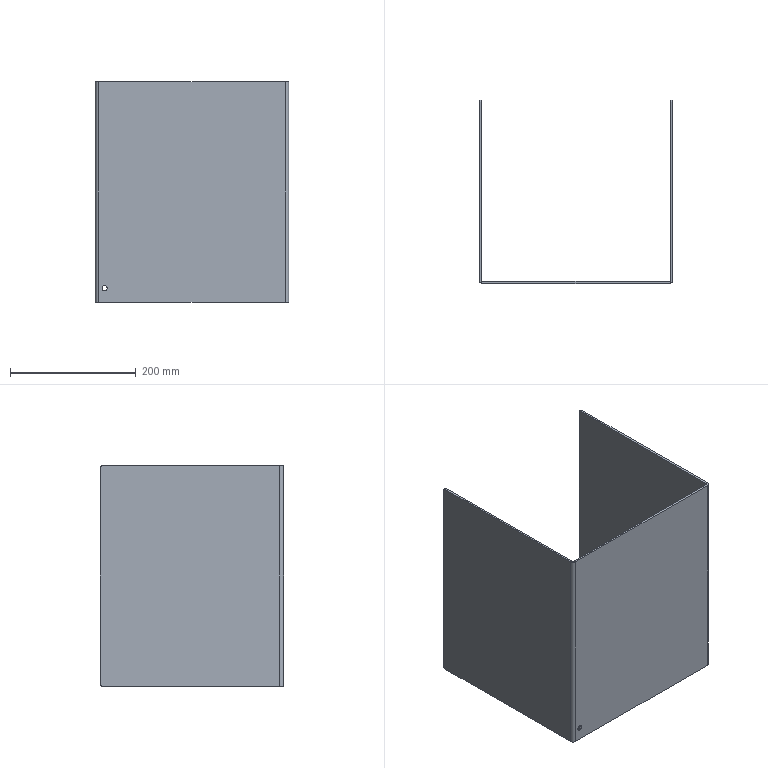Part | SolidWorks | features ICE 2, FlatPattern 1, SMBaseFlange 1, SheetMetal 1 | 1 solid | 28 faces | box 308 x 291 x 350 mm | volume 923970 mm3 | plane 18 | cylinder 10 | commonest cylinder face diameters 6 x6 8 x2 12 x2
STEP:
#1=CARTESIAN_POINT('',(15.,3.,-324.));
#2=VERTEX_POINT('',#1);
#3=CARTESIAN_POINT('',(15.,3.,-332.));
#4=VERTEX_POINT('',#3);
#5=CARTESIAN_POINT('',(15.,3.,-328.));
#6=DIRECTION('',(0.,-1.,0.));
#7=DIRECTION('',(0.,0.,-1.));
#8=AXIS2_PLACEMENT_3D('',#5,#6,#7);
#9=CIRCLE('',#8,4.);
#10=EDGE_CURVE('',#2,#4,#9,.T.);
#11=ORIENTED_EDGE('',*,*,#10,.F.);
#12=CARTESIAN_POINT('',(15.,0.,-324.));
#13=VERTEX_POINT('',#12);
#14=CARTESIAN_POINT('',(15.,10.,-324.));
#15=DIRECTION('',(0.,-1.,0.));
#16=VECTOR('',#15,1000.);
#17=LINE('',#14,#16);
#18=EDGE_CURVE('',#2,#13,#17,.T.);
#19=ORIENTED_EDGE('',*,*,#18,.T.);
#20=CARTESIAN_POINT('',(15.,0.,-332.));
#21=VERTEX_POINT('',#20);
#22=CARTESIAN_POINT('',(15.,0.,-328.));
#23=DIRECTION('',(0.,-1.,0.));
#24=DIRECTION('',(0.,0.,-1.));
#25=AXIS2_PLACEMENT_3D('',#22,#23,#24);
#26=CIRCLE('',#25,4.);
#27=EDGE_CURVE('',#13,#21,#26,.T.);
#28=ORIENTED_EDGE('',*,*,#27,.T.);
#29=CARTESIAN_POINT('',(15.,10.,-332.));
#30=DIRECTION('',(0.,-1.,0.));
#31=VECTOR('',#30,1000.);
#32=LINE('',#29,#31);
#33=EDGE_CURVE('',#4,#21,#32,.T.);
#34=ORIENTED_EDGE('',*,*,#33,.F.);
#35=EDGE_LOOP('',(#11,#19,#28,#34));
#36=FACE_OUTER_BOUND('',#35,.T.);
#37=CARTESIAN_POINT('',(15.,10.,-328.));
#38=DIRECTION('',(0.,-1.,0.));
#39=DIRECTION('',(0.,0.,-1.));
#40=AXIS2_PLACEMENT_3D('',#37,#38,#39);
#41=CYLINDRICAL_SURFACE('',#40,4.);
#42=ADVANCED_FACE('',(#36),#41,.F.);
#43=CARTESIAN_POINT('',(0.,288.,0.));
#44=VERTEX_POINT('',#43);
#45=CARTESIAN_POINT('',(0.,6.,0.));
#46=VERTEX_POINT('',#45);
#47=CARTESIAN_POINT('',(0.,0.,0.));
#48=DIRECTION('',(0.,-1.,0.));
#49=VECTOR('',#48,1000.);
#50=LINE('',#47,#49);
#51=EDGE_CURVE('',#44,#46,#50,.T.);
#52=ORIENTED_EDGE('',*,*,#51,.F.);
#53=CARTESIAN_POINT('',(0.,291.,-3.));
#54=VERTEX_POINT('',#53);
#55=CARTESIAN_POINT('',(0.,288.,-3.));
#56=DIRECTION('',(1.,0.,0.));
#57=DIRECTION('',(0.,0.,1.));
#58=AXIS2_PLACEMENT_3D('',#55,#56,#57);
#59=CIRCLE('',#58,3.);
#60=EDGE_CURVE('',#54,#44,#59,.T.);
#61=ORIENTED_EDGE('',*,*,#60,.F.);
#62=CARTESIAN_POINT('',(0.,291.,-347.));
#63=VERTEX_POINT('',#62);
#64=CARTESIAN_POINT('',(0.,291.,-350.));
#65=DIRECTION('',(0.,0.,1.));
#66=VECTOR('',#65,1000.);
#67=LINE('',#64,#66);
#68=EDGE_CURVE('',#63,#54,#67,.T.);
#69=ORIENTED_EDGE('',*,*,#68,.F.);
#70=CARTESIAN_POINT('',(0.,288.,-350.));
#71=VERTEX_POINT('',#70);
#72=CARTESIAN_POINT('',(0.,288.,-347.));
#73=DIRECTION('',(1.,0.,0.));
#74=DIRECTION('',(0.,0.,1.));
#75=AXIS2_PLACEMENT_3D('',#72,#73,#74);
#76=CIRCLE('',#75,3.);
#77=EDGE_CURVE('',#71,#63,#76,.T.);
#78=ORIENTED_EDGE('',*,*,#77,.F.);
#79=CARTESIAN_POINT('',(0.,6.,-350.));
#80=VERTEX_POINT('',#79);
#81=CARTESIAN_POINT('',(0.,0.,-350.));
#82=DIRECTION('',(0.,-1.,0.));
#83=VECTOR('',#82,1000.);
#84=LINE('',#81,#83);
#85=EDGE_CURVE('',#71,#80,#84,.T.);
#86=ORIENTED_EDGE('',*,*,#85,.T.);
#87=CARTESIAN_POINT('',(0.,6.,-350.));
#88=DIRECTION('',(0.,0.,1.));
#89=VECTOR('',#88,1000.);
#90=LINE('',#87,#89);
#91=EDGE_CURVE('',#80,#46,#90,.T.);
#92=ORIENTED_EDGE('',*,*,#91,.T.);
#93=EDGE_LOOP('',(#52,#61,#69,#78,#86,#92));
#94=FACE_OUTER_BOUND('',#93,.T.);
#95=CARTESIAN_POINT('',(0.,0.,-350.));
#96=DIRECTION('',(-1.,0.,0.));
#97=DIRECTION('',(0.,0.,1.));
#98=AXIS2_PLACEMENT_3D('',#95,#96,#97);
#99=PLANE('',#98);
#100=ADVANCED_FACE('',(#94),#99,.T.);
#101=CARTESIAN_POINT('',(3.,291.,-3.));
#102=VERTEX_POINT('',#101);
#103=CARTESIAN_POINT('',(3.,288.,0.));
#104=VERTEX_POINT('',#103);
#105=CARTESIAN_POINT('',(3.,288.,-3.));
#106=DIRECTION('',(1.,0.,0.));
#107=DIRECTION('',(0.,0.,1.));
#108=AXIS2_PLACEMENT_3D('',#105,#106,#107);
#109=CIRCLE('',#108,3.);
#110=EDGE_CURVE('',#102,#104,#109,.T.);
#111=ORIENTED_EDGE('',*,*,#110,.T.);
#112=CARTESIAN_POINT('',(3.,6.,0.));
#113=VERTEX_POINT('',#112);
#114=CARTESIAN_POINT('',(3.,0.,0.));
#115=DIRECTION('',(0.,-1.,0.));
#116=VECTOR('',#115,1000.);
#117=LINE('',#114,#116);
#118=EDGE_CURVE('',#104,#113,#117,.T.);
#119=ORIENTED_EDGE('',*,*,#118,.T.);
#120=CARTESIAN_POINT('',(3.,6.,-350.));
#121=VERTEX_POINT('',#120);
#122=CARTESIAN_POINT('',(3.,6.,-350.));
#123=DIRECTION('',(0.,0.,1.));
#124=VECTOR('',#123,1000.);
#125=LINE('',#122,#124);
#126=EDGE_CURVE('',#121,#113,#125,.T.);
#127=ORIENTED_EDGE('',*,*,#126,.F.);
#128=CARTESIAN_POINT('',(3.,288.,-350.));
#129=VERTEX_POINT('',#128);
#130=CARTESIAN_POINT('',(3.,0.,-350.));
#131=DIRECTION('',(0.,-1.,0.));
#132=VECTOR('',#131,1000.);
#133=LINE('',#130,#132);
#134=EDGE_CURVE('',#129,#121,#133,.T.);
#135=ORIENTED_EDGE('',*,*,#134,.F.);
#136=CARTESIAN_POINT('',(3.,291.,-347.));
#137=VERTEX_POINT('',#136);
#138=CARTESIAN_POINT('',(3.,288.,-347.));
#139=DIRECTION('',(1.,0.,0.));
#140=DIRECTION('',(0.,0.,1.));
#141=AXIS2_PLACEMENT_3D('',#138,#139,#140);
#142=CIRCLE('',#141,3.);
#143=EDGE_CURVE('',#129,#137,#142,.T.);
#144=ORIENTED_EDGE('',*,*,#143,.T.);
#145=CARTESIAN_POINT('',(3.,291.,-350.));
#146=DIRECTION('',(0.,0.,1.));
#147=VECTOR('',#146,1000.);
#148=LINE('',#145,#147);
#149=EDGE_CURVE('',#137,#102,#148,.T.);
#150=ORIENTED_EDGE('',*,*,#149,.T.);
#151=EDGE_LOOP('',(#111,#119,#127,#135,#144,#150));
#152=FACE_OUTER_BOUND('',#151,.T.);
#153=CARTESIAN_POINT('',(3.,0.,-350.));
#154=DIRECTION('',(-1.,0.,0.));
#155=DIRECTION('',(0.,0.,1.));
#156=AXIS2_PLACEMENT_3D('',#153,#154,#155);
#157=PLANE('',#156);
#158=ADVANCED_FACE('',(#152),#157,.F.);
#159=ORIENTED_EDGE('',*,*,#118,.F.);
#160=CARTESIAN_POINT('',(3.,288.,0.));
#161=DIRECTION('',(-1.,0.,0.));
#162=VECTOR('',#161,1000.);
#163=LINE('',#160,#162);
#164=EDGE_CURVE('',#104,#44,#163,.T.);
#165=ORIENTED_EDGE('',*,*,#164,.T.);
#166=ORIENTED_EDGE('',*,*,#51,.T.);
#167=CARTESIAN_POINT('',(0.,6.,0.));
#168=DIRECTION('',(1.,0.,0.));
#169=VECTOR('',#168,1000.);
#170=LINE('',#167,#169);
#171=EDGE_CURVE('',#46,#113,#170,.T.);
#172=ORIENTED_EDGE('',*,*,#171,.T.);
#173=EDGE_LOOP('',(#159,#165,#166,#172));
#174=FACE_OUTER_BOUND('',#173,.T.);
#175=CARTESIAN_POINT('',(6.,3.,0.));
#176=DIRECTION('',(0.,0.,1.));
#177=DIRECTION('',(1.,0.,0.));
#178=AXIS2_PLACEMENT_3D('',#175,#176,#177);
#179=PLANE('',#178);
#180=ADVANCED_FACE('',(#174),#179,.T.);
#181=CARTESIAN_POINT('',(3.,291.,-3.));
#182=DIRECTION('',(-1.,0.,0.));
#183=VECTOR('',#182,1000.);
#184=LINE('',#181,#183);
#185=EDGE_CURVE('',#102,#54,#184,.T.);
#186=ORIENTED_EDGE('',*,*,#185,.F.);
#187=ORIENTED_EDGE('',*,*,#149,.F.);
#188=CARTESIAN_POINT('',(3.,291.,-347.));
#189=DIRECTION('',(-1.,0.,0.));
#190=VECTOR('',#189,1000.);
#191=LINE('',#188,#190);
#192=EDGE_CURVE('',#137,#63,#191,.T.);
#193=ORIENTED_EDGE('',*,*,#192,.T.);
#194=ORIENTED_EDGE('',*,*,#68,.T.);
#195=EDGE_LOOP('',(#186,#187,#193,#194));
#196=FACE_OUTER_BOUND('',#195,.T.);
#197=CARTESIAN_POINT('',(0.,291.,-350.));
#198=DIRECTION('',(0.,-1.,0.));
#199=DIRECTION('',(0.,0.,-1.));
#200=AXIS2_PLACEMENT_3D('',#197,#198,#199);
#201=PLANE('',#200);
#202=ADVANCED_FACE('',(#196),#201,.F.);
#203=CARTESIAN_POINT('',(308.,291.,-347.));
#204=VERTEX_POINT('',#203);
#205=CARTESIAN_POINT('',(308.,291.,-3.));
#206=VERTEX_POINT('',#205);
#207=CARTESIAN_POINT('',(308.,291.,-350.));
#208=DIRECTION('',(0.,0.,1.));
#209=VECTOR('',#208,1000.);
#210=LINE('',#207,#209);
#211=EDGE_CURVE('',#204,#206,#210,.T.);
#212=ORIENTED_EDGE('',*,*,#211,.T.);
#213=CARTESIAN_POINT('',(308.,288.,0.));
#214=VERTEX_POINT('',#213);
#215=CARTESIAN_POINT('',(308.,288.,-3.));
#216=DIRECTION('',(-1.,0.,0.));
#217=DIRECTION('',(0.,0.,-1.));
#218=AXIS2_PLACEMENT_3D('',#215,#216,#217);
#219=CIRCLE('',#218,3.);
#220=EDGE_CURVE('',#214,#206,#219,.T.);
#221=ORIENTED_EDGE('',*,*,#220,.F.);
#222=CARTESIAN_POINT('',(308.,6.,0.));
#223=VERTEX_POINT('',#222);
#224=CARTESIAN_POINT('',(308.,0.,0.));
#225=DIRECTION('',(0.,1.,0.));
#226=VECTOR('',#225,1000.);
#227=LINE('',#224,#226);
#228=EDGE_CURVE('',#223,#214,#227,.T.);
#229=ORIENTED_EDGE('',*,*,#228,.F.);
#230=CARTESIAN_POINT('',(308.,6.,-350.));
#231=VERTEX_POINT('',#230);
#232=CARTESIAN_POINT('',(308.,6.,-350.));
#233=DIRECTION('',(0.,0.,1.));
#234=VECTOR('',#233,1000.);
#235=LINE('',#232,#234);
#236=EDGE_CURVE('',#231,#223,#235,.T.);
#237=ORIENTED_EDGE('',*,*,#236,.F.);
#238=CARTESIAN_POINT('',(308.,288.,-350.));
#239=VERTEX_POINT('',#238);
#240=CARTESIAN_POINT('',(308.,0.,-350.));
#241=DIRECTION('',(0.,1.,0.));
#242=VECTOR('',#241,1000.);
#243=LINE('',#240,#242);
#244=EDGE_CURVE('',#231,#239,#243,.T.);
#245=ORIENTED_EDGE('',*,*,#244,.T.);
#246=CARTESIAN_POINT('',(308.,288.,-347.));
#247=DIRECTION('',(-1.,0.,0.));
#248=DIRECTION('',(0.,0.,-1.));
#249=AXIS2_PLACEMENT_3D('',#246,#247,#248);
#250=CIRCLE('',#249,3.);
#251=EDGE_CURVE('',#204,#239,#250,.T.);
#252=ORIENTED_EDGE('',*,*,#251,.F.);
#253=EDGE_LOOP('',(#212,#221,#229,#237,#245,#252));
#254=FACE_OUTER_BOUND('',#253,.T.);
#255=CARTESIAN_POINT('',(308.,0.,-350.));
#256=DIRECTION('',(1.,0.,0.));
#257=DIRECTION('',(0.,0.,-1.));
#258=AXIS2_PLACEMENT_3D('',#255,#256,#257);
#259=PLANE('',#258);
#260=ADVANCED_FACE('',(#254),#259,.T.);
#261=CARTESIAN_POINT('',(305.,288.,0.));
#262=VERTEX_POINT('',#261);
#263=CARTESIAN_POINT('',(305.,291.,-3.));
#264=VERTEX_POINT('',#263);
#265=CARTESIAN_POINT('',(305.,288.,-3.));
#266=DIRECTION('',(-1.,0.,0.));
#267=DIRECTION('',(0.,0.,-1.));
#268=AXIS2_PLACEMENT_3D('',#265,#266,#267);
#269=CIRCLE('',#268,3.);
#270=EDGE_CURVE('',#262,#264,#269,.T.);
#271=ORIENTED_EDGE('',*,*,#270,.T.);
#272=CARTESIAN_POINT('',(305.,291.,-347.));
#273=VERTEX_POINT('',#272);
#274=CARTESIAN_POINT('',(305.,291.,-350.));
#275=DIRECTION('',(0.,0.,1.));
#276=VECTOR('',#275,1000.);
#277=LINE('',#274,#276);
#278=EDGE_CURVE('',#273,#264,#277,.T.);
#279=ORIENTED_EDGE('',*,*,#278,.F.);
#280=CARTESIAN_POINT('',(305.,288.,-350.));
#281=VERTEX_POINT('',#280);
#282=CARTESIAN_POINT('',(305.,288.,-347.));
#283=DIRECTION('',(-1.,0.,0.));
#284=DIRECTION('',(0.,0.,-1.));
#285=AXIS2_PLACEMENT_3D('',#282,#283,#284);
#286=CIRCLE('',#285,3.);
#287=EDGE_CURVE('',#273,#281,#286,.T.);
#288=ORIENTED_EDGE('',*,*,#287,.T.);
#289=CARTESIAN_POINT('',(305.,6.,-350.));
#290=VERTEX_POINT('',#289);
#291=CARTESIAN_POINT('',(305.,0.,-350.));
#292=DIRECTION('',(0.,1.,0.));
#293=VECTOR('',#292,1000.);
#294=LINE('',#291,#293);
#295=EDGE_CURVE('',#290,#281,#294,.T.);
#296=ORIENTED_EDGE('',*,*,#295,.F.);
#297=CARTESIAN_POINT('',(305.,6.,0.));
#298=VERTEX_POINT('',#297);
#299=CARTESIAN_POINT('',(305.,6.,-350.));
#300=DIRECTION('',(0.,0.,1.));
#301=VECTOR('',#300,1000.);
#302=LINE('',#299,#301);
#303=EDGE_CURVE('',#290,#298,#302,.T.);
#304=ORIENTED_EDGE('',*,*,#303,.T.);
#305=CARTESIAN_POINT('',(305.,0.,0.));
#306=DIRECTION('',(0.,1.,0.));
#307=VECTOR('',#306,1000.);
#308=LINE('',#305,#307);
#309=EDGE_CURVE('',#298,#262,#308,.T.);
#310=ORIENTED_EDGE('',*,*,#309,.T.);
#311=EDGE_LOOP('',(#271,#279,#288,#296,#304,#310));
#312=FACE_OUTER_BOUND('',#311,.T.);
#313=CARTESIAN_POINT('',(305.,0.,-350.));
#314=DIRECTION('',(1.,0.,0.));
#315=DIRECTION('',(0.,0.,-1.));
#316=AXIS2_PLACEMENT_3D('',#313,#314,#315);
#317=PLANE('',#316);
#318=ADVANCED_FACE('',(#312),#317,.F.);
#319=CARTESIAN_POINT('',(3.,288.,-350.));
#320=DIRECTION('',(-1.,0.,0.));
#321=VECTOR('',#320,1000.);
#322=LINE('',#319,#321);
#323=EDGE_CURVE('',#129,#71,#322,.T.);
#324=ORIENTED_EDGE('',*,*,#323,.F.);
#325=ORIENTED_EDGE('',*,*,#134,.T.);
#326=CARTESIAN_POINT('',(3.,6.,-350.));
#327=DIRECTION('',(-1.,0.,0.));
#328=VECTOR('',#327,1000.);
#329=LINE('',#326,#328);
#330=EDGE_CURVE('',#121,#80,#329,.T.);
#331=ORIENTED_EDGE('',*,*,#330,.T.);
#332=ORIENTED_EDGE('',*,*,#85,.F.);
#333=EDGE_LOOP('',(#324,#325,#331,#332));
#334=FACE_OUTER_BOUND('',#333,.T.);
#335=CARTESIAN_POINT('',(302.,6.,-350.));
#336=DIRECTION('',(0.,0.,1.));
#337=DIRECTION('',(1.,0.,0.));
#338=AXIS2_PLACEMENT_3D('',#335,#336,#337);
#339=PLANE('',#338);
#340=ADVANCED_FACE('',(#334),#339,.F.);
#341=ORIENTED_EDGE('',*,*,#295,.T.);
#342=CARTESIAN_POINT('',(305.,288.,-350.));
#343=DIRECTION('',(1.,0.,0.));
#344=VECTOR('',#343,1000.);
#345=LINE('',#342,#344);
#346=EDGE_CURVE('',#281,#239,#345,.T.);
#347=ORIENTED_EDGE('',*,*,#346,.T.);
#348=ORIENTED_EDGE('',*,*,#244,.F.);
#349=CARTESIAN_POINT('',(308.,6.,-350.));
#350=DIRECTION('',(-1.,0.,0.));
#351=VECTOR('',#350,1000.);
#352=LINE('',#349,#351);
#353=EDGE_CURVE('',#231,#290,#352,.T.);
#354=ORIENTED_EDGE('',*,*,#353,.T.);
#355=EDGE_LOOP('',(#341,#347,#348,#354));
#356=FACE_OUTER_BOUND('',#355,.T.);
#357=CARTESIAN_POINT('',(302.,3.,-350.));
#358=DIRECTION('',(0.,0.,-1.));
#359=DIRECTION('',(-1.,0.,0.));
#360=AXIS2_PLACEMENT_3D('',#357,#358,#359);
#361=PLANE('',#360);
#362=ADVANCED_FACE('',(#356),#361,.T.);
#363=ORIENTED_EDGE('',*,*,#278,.T.);
#364=CARTESIAN_POINT('',(305.,291.,-3.));
#365=DIRECTION('',(1.,0.,0.));
#366=VECTOR('',#365,1000.);
#367=LINE('',#364,#366);
#368=EDGE_CURVE('',#264,#206,#367,.T.);
#369=ORIENTED_EDGE('',*,*,#368,.T.);
#370=ORIENTED_EDGE('',*,*,#211,.F.);
#371=CARTESIAN_POINT('',(305.,291.,-347.));
#372=DIRECTION('',(1.,0.,0.));
#373=VECTOR('',#372,1000.);
#374=LINE('',#371,#373);
#375=EDGE_CURVE('',#273,#204,#374,.T.);
#376=ORIENTED_EDGE('',*,*,#375,.F.);
#377=EDGE_LOOP('',(#363,#369,#370,#376));
#378=FACE_OUTER_BOUND('',#377,.T.);
#379=CARTESIAN_POINT('',(305.,291.,-350.));
#380=DIRECTION('',(0.,-1.,0.));
#381=DIRECTION('',(0.,0.,-1.));
#382=AXIS2_PLACEMENT_3D('',#379,#380,#381);
#383=PLANE('',#382);
#384=ADVANCED_FACE('',(#378),#383,.F.);
#385=CARTESIAN_POINT('',(6.,0.,-350.));
#386=VERTEX_POINT('',#385);
#387=CARTESIAN_POINT('',(6.,3.,-350.));
#388=VERTEX_POINT('',#387);
#389=CARTESIAN_POINT('',(6.,0.,-350.));
#390=DIRECTION('',(0.,1.,0.));
#391=VECTOR('',#390,1000.);
#392=LINE('',#389,#391);
#393=EDGE_CURVE('',#386,#388,#392,.T.);
#394=ORIENTED_EDGE('',*,*,#393,.F.);
#395=CARTESIAN_POINT('',(6.,6.,-350.));
#396=DIRECTION('',(0.,0.,1.));
#397=DIRECTION('',(-1.,0.,0.));
#398=AXIS2_PLACEMENT_3D('',#395,#396,#397);
#399=CIRCLE('',#398,6.);
#400=EDGE_CURVE('',#80,#386,#399,.T.);
#401=ORIENTED_EDGE('',*,*,#400,.F.);
#402=ORIENTED_EDGE('',*,*,#330,.F.);
#403=CARTESIAN_POINT('',(6.,6.,-350.));
#404=DIRECTION('',(0.,0.,1.));
#405=DIRECTION('',(1.,0.,0.));
#406=AXIS2_PLACEMENT_3D('',#403,#404,#405);
#407=CIRCLE('',#406,3.);
#408=EDGE_CURVE('',#121,#388,#407,.T.);
#409=ORIENTED_EDGE('',*,*,#408,.T.);
#410=EDGE_LOOP('',(#394,#401,#402,#409));
#411=FACE_OUTER_BOUND('',#410,.T.);
#412=CARTESIAN_POINT('',(6.,0.,-350.));
#413=DIRECTION('',(0.,0.,-1.));
#414=DIRECTION('',(-1.,0.,0.));
#415=AXIS2_PLACEMENT_3D('',#412,#413,#414);
#416=PLANE('',#415);
#417=ADVANCED_FACE('',(#411),#416,.T.);
#418=CARTESIAN_POINT('',(302.,0.,-350.));
#419=VERTEX_POINT('',#418);
#420=CARTESIAN_POINT('',(0.,0.,-350.));
#421=DIRECTION('',(1.,0.,0.));
#422=VECTOR('',#421,1000.);
#423=LINE('',#420,#422);
#424=EDGE_CURVE('',#386,#419,#423,.T.);
#425=ORIENTED_EDGE('',*,*,#424,.F.);
#426=ORIENTED_EDGE('',*,*,#393,.T.);
#427=CARTESIAN_POINT('',(302.,3.,-350.));
#428=VERTEX_POINT('',#427);
#429=CARTESIAN_POINT('',(0.,3.,-350.));
#430=DIRECTION('',(1.,0.,0.));
#431=VECTOR('',#430,1000.);
#432=LINE('',#429,#431);
#433=EDGE_CURVE('',#388,#428,#432,.T.);
#434=ORIENTED_EDGE('',*,*,#433,.T.);
#435=CARTESIAN_POINT('',(302.,3.,-350.));
#436=DIRECTION('',(0.,-1.,0.));
#437=VECTOR('',#436,1000.);
#438=LINE('',#435,#437);
#439=EDGE_CURVE('',#428,#419,#438,.T.);
#440=ORIENTED_EDGE('',*,*,#439,.T.);
#441=EDGE_LOOP('',(#425,#426,#434,#440));
#442=FACE_OUTER_BOUND('',#441,.T.);
#443=CARTESIAN_POINT('',(3.,6.,-350.));
#444=DIRECTION('',(0.,0.,-1.));
#445=DIRECTION('',(-1.,0.,0.));
#446=AXIS2_PLACEMENT_3D('',#443,#444,#445);
#447=PLANE('',#446);
#448=ADVANCED_FACE('',(#442),#447,.T.);
#449=ORIENTED_EDGE('',*,*,#171,.F.);
#450=CARTESIAN_POINT('',(6.,0.,0.));
#451=VERTEX_POINT('',#450);
#452=CARTESIAN_POINT('',(6.,6.,0.));
#453=DIRECTION('',(0.,0.,1.));
#454=DIRECTION('',(-1.,0.,0.));
#455=AXIS2_PLACEMENT_3D('',#452,#453,#454);
#456=CIRCLE('',#455,6.);
#457=EDGE_CURVE('',#46,#451,#456,.T.);
#458=ORIENTED_EDGE('',*,*,#457,.T.);
#459=CARTESIAN_POINT('',(6.,3.,0.));
#460=VERTEX_POINT('',#459);
#461=CARTESIAN_POINT('',(6.,3.,0.));
#462=DIRECTION('',(0.,-1.,0.));
#463=VECTOR('',#462,1000.);
#464=LINE('',#461,#463);
#465=EDGE_CURVE('',#460,#451,#464,.T.);
#466=ORIENTED_EDGE('',*,*,#465,.F.);
#467=CARTESIAN_POINT('',(6.,6.,0.));
#468=DIRECTION('',(0.,0.,1.));
#469=DIRECTION('',(1.,0.,0.));
#470=AXIS2_PLACEMENT_3D('',#467,#468,#469);
#471=CIRCLE('',#470,3.);
#472=EDGE_CURVE('',#113,#460,#471,.T.);
#473=ORIENTED_EDGE('',*,*,#472,.F.);
#474=EDGE_LOOP('',(#449,#458,#466,#473));
#475=FACE_OUTER_BOUND('',#474,.T.);
#476=CARTESIAN_POINT('',(0.,6.,0.));
#477=DIRECTION('',(0.,0.,1.));
#478=DIRECTION('',(1.,0.,0.));
#479=AXIS2_PLACEMENT_3D('',#476,#477,#478);
#480=PLANE('',#479);
#481=ADVANCED_FACE('',(#475),#480,.T.);
#482=ORIENTED_EDGE('',*,*,#353,.F.);
#483=CARTESIAN_POINT('',(302.,6.,-350.));
#484=DIRECTION('',(0.,0.,1.));
#485=DIRECTION('',(-1.,0.,0.));
#486=AXIS2_PLACEMENT_3D('',#483,#484,#485);
#487=CIRCLE('',#486,6.);
#488=EDGE_CURVE('',#419,#231,#487,.T.);
#489=ORIENTED_EDGE('',*,*,#488,.F.);
#490=ORIENTED_EDGE('',*,*,#439,.F.);
#491=CARTESIAN_POINT('',(302.,6.,-350.));
#492=DIRECTION('',(0.,0.,1.));
#493=DIRECTION('',(1.,0.,0.));
#494=AXIS2_PLACEMENT_3D('',#491,#492,#493);
#495=CIRCLE('',#494,3.);
#496=EDGE_CURVE('',#428,#290,#495,.T.);
#497=ORIENTED_EDGE('',*,*,#496,.T.);
#498=EDGE_LOOP('',(#482,#489,#490,#497));
#499=FACE_OUTER_BOUND('',#498,.T.);
#500=CARTESIAN_POINT('',(308.,6.,-350.));
#501=DIRECTION('',(0.,0.,-1.));
#502=DIRECTION('',(-1.,0.,0.));
#503=AXIS2_PLACEMENT_3D('',#500,#501,#502);
#504=PLANE('',#503);
#505=ADVANCED_FACE('',(#499),#504,.T.);
#506=CARTESIAN_POINT('',(302.,0.,0.));
#507=VERTEX_POINT('',#506);
#508=CARTESIAN_POINT('',(302.,3.,0.));
#509=VERTEX_POINT('',#508);
#510=CARTESIAN_POINT('',(302.,0.,0.));
#511=DIRECTION('',(0.,1.,0.));
#512=VECTOR('',#511,1000.);
#513=LINE('',#510,#512);
#514=EDGE_CURVE('',#507,#509,#513,.T.);
#515=ORIENTED_EDGE('',*,*,#514,.F.);
#516=CARTESIAN_POINT('',(302.,6.,0.));
#517=DIRECTION('',(0.,0.,1.));
#518=DIRECTION('',(-1.,0.,0.));
#519=AXIS2_PLACEMENT_3D('',#516,#517,#518);
#520=CIRCLE('',#519,6.);
#521=EDGE_CURVE('',#507,#223,#520,.T.);
#522=ORIENTED_EDGE('',*,*,#521,.T.);
#523=CARTESIAN_POINT('',(305.,6.,0.));
#524=DIRECTION('',(1.,0.,0.));
#525=VECTOR('',#524,1000.);
#526=LINE('',#523,#525);
#527=EDGE_CURVE('',#298,#223,#526,.T.);
#528=ORIENTED_EDGE('',*,*,#527,.F.);
#529=CARTESIAN_POINT('',(302.,6.,0.));
#530=DIRECTION('',(0.,0.,1.));
#531=DIRECTION('',(1.,0.,0.));
#532=AXIS2_PLACEMENT_3D('',#529,#530,#531);
#533=CIRCLE('',#532,3.);
#534=EDGE_CURVE('',#509,#298,#533,.T.);
#535=ORIENTED_EDGE('',*,*,#534,.F.);
#536=EDGE_LOOP('',(#515,#522,#528,#535));
#537=FACE_OUTER_BOUND('',#536,.T.);
#538=CARTESIAN_POINT('',(302.,0.,0.));
#539=DIRECTION('',(0.,0.,1.));
#540=DIRECTION('',(1.,0.,0.));
#541=AXIS2_PLACEMENT_3D('',#538,#539,#540);
#542=PLANE('',#541);
#543=ADVANCED_FACE('',(#537),#542,.T.);
#544=CARTESIAN_POINT('',(0.,0.,0.));
#545=DIRECTION('',(1.,0.,0.));
#546=VECTOR('',#545,1000.);
#547=LINE('',#544,#546);
#548=EDGE_CURVE('',#451,#507,#547,.T.);
#549=ORIENTED_EDGE('',*,*,#548,.T.);
#550=ORIENTED_EDGE('',*,*,#514,.T.);
#551=CARTESIAN_POINT('',(0.,3.,0.));
#552=DIRECTION('',(1.,0.,0.));
#553=VECTOR('',#552,1000.);
#554=LINE('',#551,#553);
#555=EDGE_CURVE('',#460,#509,#554,.T.);
#556=ORIENTED_EDGE('',*,*,#555,.F.);
#557=ORIENTED_EDGE('',*,*,#465,.T.);
#558=EDGE_LOOP('',(#549,#550,#556,#557));
#559=FACE_OUTER_BOUND('',#558,.T.);
#560=CARTESIAN_POINT('',(305.,6.,0.));
#561=DIRECTION('',(0.,0.,1.));
#562=DIRECTION('',(1.,0.,0.));
#563=AXIS2_PLACEMENT_3D('',#560,#561,#562);
#564=PLANE('',#563);
#565=ADVANCED_FACE('',(#559),#564,.T.);
#566=ORIENTED_EDGE('',*,*,#521,.F.);
#567=CARTESIAN_POINT('',(302.,0.,-350.));
#568=DIRECTION('',(0.,0.,1.));
#569=VECTOR('',#568,1000.);
#570=LINE('',#567,#569);
#571=EDGE_CURVE('',#419,#507,#570,.T.);
#572=ORIENTED_EDGE('',*,*,#571,.F.);
#573=ORIENTED_EDGE('',*,*,#488,.T.);
#574=ORIENTED_EDGE('',*,*,#236,.T.);
#575=EDGE_LOOP('',(#566,#572,#573,#574));
#576=FACE_OUTER_BOUND('',#575,.T.);
#577=CARTESIAN_POINT('',(302.,6.,-350.));
#578=DIRECTION('',(0.,0.,1.));
#579=DIRECTION('',(1.,0.,0.));
#580=AXIS2_PLACEMENT_3D('',#577,#578,#579);
#581=CYLINDRICAL_SURFACE('',#580,6.);
#582=ADVANCED_FACE('',(#576),#581,.T.);
#583=CARTESIAN_POINT('',(15.,0.,-328.));
#584=DIRECTION('',(0.,-1.,0.));
#585=DIRECTION('',(0.,0.,-1.));
#586=AXIS2_PLACEMENT_3D('',#583,#584,#585);
#587=CIRCLE('',#586,4.);
#588=EDGE_CURVE('',#21,#13,#587,.T.);
#589=ORIENTED_EDGE('',*,*,#588,.F.);
#590=ORIENTED_EDGE('',*,*,#27,.F.);
#591=EDGE_LOOP('',(#589,#590));
#592=FACE_BOUND('',#591,.T.);
#593=ORIENTED_EDGE('',*,*,#548,.F.);
#594=CARTESIAN_POINT('',(6.,0.,-350.));
#595=DIRECTION('',(0.,0.,1.));
#596=VECTOR('',#595,1000.);
#597=LINE('',#594,#596);
#598=EDGE_CURVE('',#386,#451,#597,.T.);
#599=ORIENTED_EDGE('',*,*,#598,.F.);
#600=ORIENTED_EDGE('',*,*,#424,.T.);
#601=ORIENTED_EDGE('',*,*,#571,.T.);
#602=EDGE_LOOP('',(#593,#599,#600,#601));
#603=FACE_OUTER_BOUND('',#602,.T.);
#604=CARTESIAN_POINT('',(0.,0.,-350.));
#605=DIRECTION('',(0.,-1.,0.));
#606=DIRECTION('',(0.,0.,-1.));
#607=AXIS2_PLACEMENT_3D('',#604,#605,#606);
#608=PLANE('',#607);
#609=ADVANCED_FACE('',(#592,#603),#608,.T.);
#610=ORIENTED_EDGE('',*,*,#457,.F.);
#611=ORIENTED_EDGE('',*,*,#91,.F.);
#612=ORIENTED_EDGE('',*,*,#400,.T.);
#613=ORIENTED_EDGE('',*,*,#598,.T.);
#614=EDGE_LOOP('',(#610,#611,#612,#613));
#615=FACE_OUTER_BOUND('',#614,.T.);
#616=CARTESIAN_POINT('',(6.,6.,-350.));
#617=DIRECTION('',(0.,0.,1.));
#618=DIRECTION('',(1.,0.,0.));
#619=AXIS2_PLACEMENT_3D('',#616,#617,#618);
#620=CYLINDRICAL_SURFACE('',#619,6.);
#621=ADVANCED_FACE('',(#615),#620,.T.);
#622=ORIENTED_EDGE('',*,*,#472,.T.);
#623=CARTESIAN_POINT('',(6.,3.,-350.));
#624=DIRECTION('',(0.,0.,1.));
#625=VECTOR('',#624,1000.);
#626=LINE('',#623,#625);
#627=EDGE_CURVE('',#388,#460,#626,.T.);
#628=ORIENTED_EDGE('',*,*,#627,.F.);
#629=ORIENTED_EDGE('',*,*,#408,.F.);
#630=ORIENTED_EDGE('',*,*,#126,.T.);
#631=EDGE_LOOP('',(#622,#628,#629,#630));
#632=FACE_OUTER_BOUND('',#631,.T.);
#633=CARTESIAN_POINT('',(6.,6.,-350.));
#634=DIRECTION('',(0.,0.,1.));
#635=DIRECTION('',(1.,0.,0.));
#636=AXIS2_PLACEMENT_3D('',#633,#634,#635);
#637=CYLINDRICAL_SURFACE('',#636,3.);
#638=ADVANCED_FACE('',(#632),#637,.F.);
#639=CARTESIAN_POINT('',(15.,3.,-328.));
#640=DIRECTION('',(0.,-1.,0.));
#641=DIRECTION('',(0.,0.,-1.));
#642=AXIS2_PLACEMENT_3D('',#639,#640,#641);
#643=CIRCLE('',#642,4.);
#644=EDGE_CURVE('',#4,#2,#643,.T.);
#645=ORIENTED_EDGE('',*,*,#644,.T.);
#646=ORIENTED_EDGE('',*,*,#10,.T.);
#647=EDGE_LOOP('',(#645,#646));
#648=FACE_BOUND('',#647,.T.);
#649=ORIENTED_EDGE('',*,*,#555,.T.);
#650=CARTESIAN_POINT('',(302.,3.,-350.));
#651=DIRECTION('',(0.,0.,1.));
#652=VECTOR('',#651,1000.);
#653=LINE('',#650,#652);
#654=EDGE_CURVE('',#428,#509,#653,.T.);
#655=ORIENTED_EDGE('',*,*,#654,.F.);
#656=ORIENTED_EDGE('',*,*,#433,.F.);
#657=ORIENTED_EDGE('',*,*,#627,.T.);
#658=EDGE_LOOP('',(#649,#655,#656,#657));
#659=FACE_OUTER_BOUND('',#658,.T.);
#660=CARTESIAN_POINT('',(0.,3.,-350.));
#661=DIRECTION('',(0.,-1.,0.));
#662=DIRECTION('',(0.,0.,-1.));
#663=AXIS2_PLACEMENT_3D('',#660,#661,#662);
#664=PLANE('',#663);
#665=ADVANCED_FACE('',(#648,#659),#664,.F.);
#666=ORIENTED_EDGE('',*,*,#534,.T.);
#667=ORIENTED_EDGE('',*,*,#303,.F.);
#668=ORIENTED_EDGE('',*,*,#496,.F.);
#669=ORIENTED_EDGE('',*,*,#654,.T.);
#670=EDGE_LOOP('',(#666,#667,#668,#669));
#671=FACE_OUTER_BOUND('',#670,.T.);
#672=CARTESIAN_POINT('',(302.,6.,-350.));
#673=DIRECTION('',(0.,0.,1.));
#674=DIRECTION('',(1.,0.,0.));
#675=AXIS2_PLACEMENT_3D('',#672,#673,#674);
#676=CYLINDRICAL_SURFACE('',#675,3.);
#677=ADVANCED_FACE('',(#671),#676,.F.);
#678=CARTESIAN_POINT('',(305.,288.,0.));
#679=DIRECTION('',(1.,0.,0.));
#680=VECTOR('',#679,1000.);
#681=LINE('',#678,#680);
#682=EDGE_CURVE('',#262,#214,#681,.T.);
#683=ORIENTED_EDGE('',*,*,#682,.F.);
#684=ORIENTED_EDGE('',*,*,#309,.F.);
#685=ORIENTED_EDGE('',*,*,#527,.T.);
#686=ORIENTED_EDGE('',*,*,#228,.T.);
#687=EDGE_LOOP('',(#683,#684,#685,#686));
#688=FACE_OUTER_BOUND('',#687,.T.);
#689=CARTESIAN_POINT('',(302.,6.,0.));
#690=DIRECTION('',(0.,0.,1.));
#691=DIRECTION('',(1.,0.,0.));
#692=AXIS2_PLACEMENT_3D('',#689,#690,#691);
#693=PLANE('',#692);
#694=ADVANCED_FACE('',(#688),#693,.T.);
#695=ORIENTED_EDGE('',*,*,#18,.F.);
#696=ORIENTED_EDGE('',*,*,#644,.F.);
#697=ORIENTED_EDGE('',*,*,#33,.T.);
#698=ORIENTED_EDGE('',*,*,#588,.T.);
#699=EDGE_LOOP('',(#695,#696,#697,#698));
#700=FACE_OUTER_BOUND('',#699,.T.);
#701=CARTESIAN_POINT('',(15.,10.,-328.));
#702=DIRECTION('',(0.,-1.,0.));
#703=DIRECTION('',(0.,0.,-1.));
#704=AXIS2_PLACEMENT_3D('',#701,#702,#703);
#705=CYLINDRICAL_SURFACE('',#704,4.);
#706=ADVANCED_FACE('',(#700),#705,.F.);
#707=ORIENTED_EDGE('',*,*,#346,.F.);
#708=ORIENTED_EDGE('',*,*,#287,.F.);
#709=ORIENTED_EDGE('',*,*,#375,.T.);
#710=ORIENTED_EDGE('',*,*,#251,.T.);
#711=EDGE_LOOP('',(#707,#708,#709,#710));
#712=FACE_OUTER_BOUND('',#711,.T.);
#713=CARTESIAN_POINT('',(305.,288.,-347.));
#714=DIRECTION('',(1.,0.,0.));
#715=DIRECTION('',(0.,0.,-1.));
#716=AXIS2_PLACEMENT_3D('',#713,#714,#715);
#717=CYLINDRICAL_SURFACE('',#716,3.);
#718=ADVANCED_FACE('',(#712),#717,.T.);
#719=ORIENTED_EDGE('',*,*,#192,.F.);
#720=ORIENTED_EDGE('',*,*,#143,.F.);
#721=ORIENTED_EDGE('',*,*,#323,.T.);
#722=ORIENTED_EDGE('',*,*,#77,.T.);
#723=EDGE_LOOP('',(#719,#720,#721,#722));
#724=FACE_OUTER_BOUND('',#723,.T.);
#725=CARTESIAN_POINT('',(3.,288.,-347.));
#726=DIRECTION('',(-1.,0.,0.));
#727=DIRECTION('',(0.,0.,1.));
#728=AXIS2_PLACEMENT_3D('',#725,#726,#727);
#729=CYLINDRICAL_SURFACE('',#728,3.);
#730=ADVANCED_FACE('',(#724),#729,.T.);
#731=ORIENTED_EDGE('',*,*,#368,.F.);
#732=ORIENTED_EDGE('',*,*,#270,.F.);
#733=ORIENTED_EDGE('',*,*,#682,.T.);
#734=ORIENTED_EDGE('',*,*,#220,.T.);
#735=EDGE_LOOP('',(#731,#732,#733,#734));
#736=FACE_OUTER_BOUND('',#735,.T.);
#737=CARTESIAN_POINT('',(305.,288.,-3.));
#738=DIRECTION('',(1.,0.,0.));
#739=DIRECTION('',(0.,0.,-1.));
#740=AXIS2_PLACEMENT_3D('',#737,#738,#739);
#741=CYLINDRICAL_SURFACE('',#740,3.);
#742=ADVANCED_FACE('',(#736),#741,.T.);
#743=ORIENTED_EDGE('',*,*,#164,.F.);
#744=ORIENTED_EDGE('',*,*,#110,.F.);
#745=ORIENTED_EDGE('',*,*,#185,.T.);
#746=ORIENTED_EDGE('',*,*,#60,.T.);
#747=EDGE_LOOP('',(#743,#744,#745,#746));
#748=FACE_OUTER_BOUND('',#747,.T.);
#749=CARTESIAN_POINT('',(3.,288.,-3.));
#750=DIRECTION('',(-1.,0.,0.));
#751=DIRECTION('',(0.,0.,1.));
#752=AXIS2_PLACEMENT_3D('',#749,#750,#751);
#753=CYLINDRICAL_SURFACE('',#752,3.);
#754=ADVANCED_FACE('',(#748),#753,.T.);
#755=CLOSED_SHELL('',(#42,#100,#158,#180,#202,#260,#318,#340,#362,#384,#417,#448,#481,#505,#543,#565,#582,#609,#621,#638,#665,#677,#694,#706,#718,#730,#742,#754));
#756=MANIFOLD_SOLID_BREP('',#755);
#757=CARTESIAN_POINT('',(0.,0.,0.));
#758=DIRECTION('',(0.,0.,1.));
#759=DIRECTION('',(1.,0.,0.));
#760=AXIS2_PLACEMENT_3D('',#757,#758,#759);
#761=(LENGTH_UNIT()NAMED_UNIT(*)SI_UNIT(.MILLI.,.METRE.));
#762=UNCERTAINTY_MEASURE_WITH_UNIT(LENGTH_MEASURE(0.00001),#761,'','');
#763=(NAMED_UNIT(*)PLANE_ANGLE_UNIT()SI_UNIT($,.RADIAN.));
#764=(NAMED_UNIT(*)SI_UNIT($,.STERADIAN.)SOLID_ANGLE_UNIT());
#765=(GEOMETRIC_REPRESENTATION_CONTEXT(3)GLOBAL_UNCERTAINTY_ASSIGNED_CONTEXT((#762))GLOBAL_UNIT_ASSIGNED_CONTEXT((#761,#763,#764))REPRESENTATION_CONTEXT('',''));
#766=ADVANCED_BREP_SHAPE_REPRESENTATION('',(#756,#760),#765);